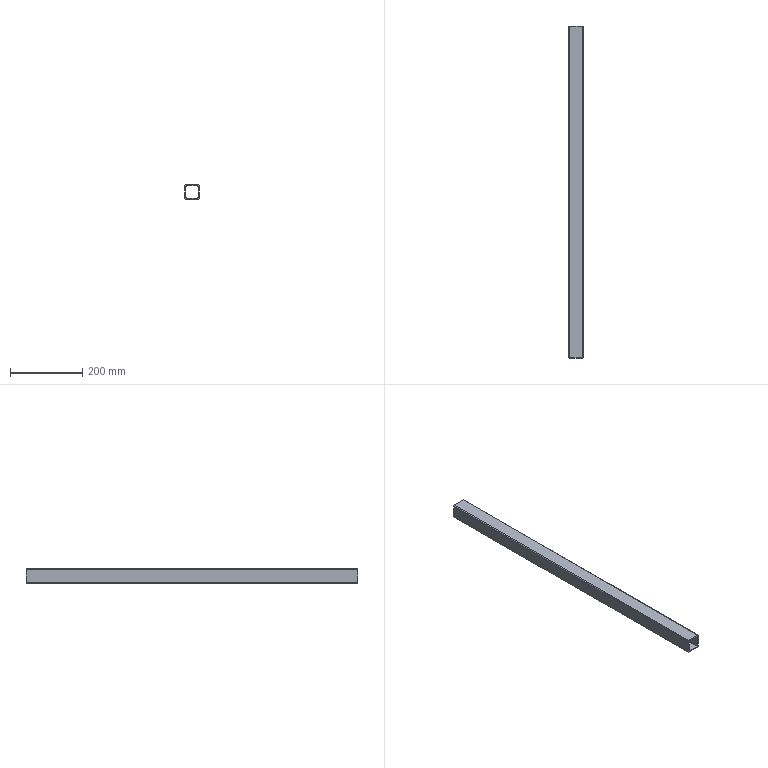Part | STEP file | SynoNew-0304-043 | 1 solid | 18 faces | box 40 x 920 x 40 mm | volume 408480 mm3 | plane 10 | cylinder 8 | commonest cylinder face diameters 4 x8
STEP:
#1=CARTESIAN_POINT('',(-18.,-460.,0.));
#2=VERTEX_POINT('',#1);
#3=CARTESIAN_POINT('',(-20.,-460.,2.));
#4=VERTEX_POINT('',#3);
#5=CARTESIAN_POINT('',(-18.,-460.,2.));
#6=DIRECTION('',(0.,1.,0.));
#7=DIRECTION('',(-0.7071,0.,-0.7071));
#8=AXIS2_PLACEMENT_3D('',#5,#6,#7);
#9=CIRCLE('',#8,2.);
#10=EDGE_CURVE('',#2,#4,#9,.T.);
#11=ORIENTED_EDGE('',*,*,#10,.T.);
#12=CARTESIAN_POINT('',(-20.,460.,2.));
#13=VERTEX_POINT('',#12);
#14=CARTESIAN_POINT('',(-20.,230.,2.));
#15=DIRECTION('',(0.,1.,0.));
#16=VECTOR('',#15,10.);
#17=LINE('',#14,#16);
#18=EDGE_CURVE('',#4,#13,#17,.T.);
#19=ORIENTED_EDGE('',*,*,#18,.T.);
#20=CARTESIAN_POINT('',(-18.,460.,0.));
#21=VERTEX_POINT('',#20);
#22=CARTESIAN_POINT('',(-18.,460.,2.));
#23=DIRECTION('',(0.,-1.,0.));
#24=DIRECTION('',(-0.7071,0.,-0.7071));
#25=AXIS2_PLACEMENT_3D('',#22,#23,#24);
#26=CIRCLE('',#25,2.);
#27=EDGE_CURVE('',#13,#21,#26,.T.);
#28=ORIENTED_EDGE('',*,*,#27,.T.);
#29=CARTESIAN_POINT('',(-18.,230.,0.));
#30=DIRECTION('',(0.,-1.,0.));
#31=VECTOR('',#30,10.);
#32=LINE('',#29,#31);
#33=EDGE_CURVE('',#21,#2,#32,.T.);
#34=ORIENTED_EDGE('',*,*,#33,.T.);
#35=EDGE_LOOP('',(#11,#19,#28,#34));
#36=FACE_OUTER_BOUND('',#35,.T.);
#37=CARTESIAN_POINT('',(-18.,230.,2.));
#38=DIRECTION('',(0.,-1.,0.));
#39=DIRECTION('',(-0.7071,0.,-0.7071));
#40=AXIS2_PLACEMENT_3D('',#37,#38,#39);
#41=CYLINDRICAL_SURFACE('',#40,2.);
#42=ADVANCED_FACE('',(#36),#41,.T.);
#43=ORIENTED_EDGE('',*,*,#33,.F.);
#44=CARTESIAN_POINT('',(18.,460.,0.));
#45=VERTEX_POINT('',#44);
#46=CARTESIAN_POINT('',(20.,460.,0.));
#47=DIRECTION('',(-1.,0.,0.));
#48=VECTOR('',#47,10.);
#49=LINE('',#46,#48);
#50=EDGE_CURVE('',#45,#21,#49,.T.);
#51=ORIENTED_EDGE('',*,*,#50,.F.);
#52=CARTESIAN_POINT('',(18.,-460.,0.));
#53=VERTEX_POINT('',#52);
#54=CARTESIAN_POINT('',(18.,-230.,0.));
#55=DIRECTION('',(0.,1.,0.));
#56=VECTOR('',#55,10.);
#57=LINE('',#54,#56);
#58=EDGE_CURVE('',#53,#45,#57,.T.);
#59=ORIENTED_EDGE('',*,*,#58,.F.);
#60=CARTESIAN_POINT('',(-20.,-460.,0.));
#61=DIRECTION('',(1.,0.,0.));
#62=VECTOR('',#61,10.);
#63=LINE('',#60,#62);
#64=EDGE_CURVE('',#2,#53,#63,.T.);
#65=ORIENTED_EDGE('',*,*,#64,.F.);
#66=EDGE_LOOP('',(#43,#51,#59,#65));
#67=FACE_OUTER_BOUND('',#66,.T.);
#68=CARTESIAN_POINT('',(0.,0.,0.));
#69=DIRECTION('',(0.,0.,1.));
#70=DIRECTION('',(1.,0.,0.));
#71=AXIS2_PLACEMENT_3D('',#68,#69,#70);
#72=PLANE('',#71);
#73=ADVANCED_FACE('',(#67),#72,.F.);
#74=ORIENTED_EDGE('',*,*,#27,.F.);
#75=CARTESIAN_POINT('',(-20.,460.,38.));
#76=VERTEX_POINT('',#75);
#77=CARTESIAN_POINT('',(-20.,460.,0.));
#78=DIRECTION('',(0.,0.,1.));
#79=VECTOR('',#78,10.);
#80=LINE('',#77,#79);
#81=EDGE_CURVE('',#13,#76,#80,.T.);
#82=ORIENTED_EDGE('',*,*,#81,.T.);
#83=CARTESIAN_POINT('',(-18.,460.,40.));
#84=VERTEX_POINT('',#83);
#85=CARTESIAN_POINT('',(-18.,460.,38.));
#86=DIRECTION('',(0.,-1.,0.));
#87=DIRECTION('',(-0.7071,0.,0.7071));
#88=AXIS2_PLACEMENT_3D('',#85,#86,#87);
#89=CIRCLE('',#88,2.);
#90=EDGE_CURVE('',#84,#76,#89,.T.);
#91=ORIENTED_EDGE('',*,*,#90,.F.);
#92=CARTESIAN_POINT('',(18.,460.,40.));
#93=VERTEX_POINT('',#92);
#94=CARTESIAN_POINT('',(20.,460.,40.));
#95=DIRECTION('',(-1.,0.,0.));
#96=VECTOR('',#95,10.);
#97=LINE('',#94,#96);
#98=EDGE_CURVE('',#93,#84,#97,.T.);
#99=ORIENTED_EDGE('',*,*,#98,.F.);
#100=CARTESIAN_POINT('',(20.,460.,38.));
#101=VERTEX_POINT('',#100);
#102=CARTESIAN_POINT('',(18.,460.,38.));
#103=DIRECTION('',(0.,-1.,0.));
#104=DIRECTION('',(0.7071,0.,0.7071));
#105=AXIS2_PLACEMENT_3D('',#102,#103,#104);
#106=CIRCLE('',#105,2.);
#107=EDGE_CURVE('',#101,#93,#106,.T.);
#108=ORIENTED_EDGE('',*,*,#107,.F.);
#109=CARTESIAN_POINT('',(20.,460.,2.));
#110=VERTEX_POINT('',#109);
#111=CARTESIAN_POINT('',(20.,460.,0.));
#112=DIRECTION('',(0.,0.,1.));
#113=VECTOR('',#112,10.);
#114=LINE('',#111,#113);
#115=EDGE_CURVE('',#110,#101,#114,.T.);
#116=ORIENTED_EDGE('',*,*,#115,.F.);
#117=CARTESIAN_POINT('',(18.,460.,2.));
#118=DIRECTION('',(0.,-1.,0.));
#119=DIRECTION('',(0.7071,0.,-0.7071));
#120=AXIS2_PLACEMENT_3D('',#117,#118,#119);
#121=CIRCLE('',#120,2.);
#122=EDGE_CURVE('',#45,#110,#121,.T.);
#123=ORIENTED_EDGE('',*,*,#122,.F.);
#124=ORIENTED_EDGE('',*,*,#50,.T.);
#125=EDGE_LOOP('',(#74,#82,#91,#99,#108,#116,#123,#124));
#126=FACE_OUTER_BOUND('',#125,.T.);
#127=CARTESIAN_POINT('',(17.,460.,5.));
#128=VERTEX_POINT('',#127);
#129=CARTESIAN_POINT('',(17.,460.,35.));
#130=VERTEX_POINT('',#129);
#131=CARTESIAN_POINT('',(17.,460.,1.5));
#132=DIRECTION('',(0.,0.,1.));
#133=VECTOR('',#132,10.);
#134=LINE('',#131,#133);
#135=EDGE_CURVE('',#128,#130,#134,.T.);
#136=ORIENTED_EDGE('',*,*,#135,.T.);
#137=CARTESIAN_POINT('',(15.,460.,37.));
#138=VERTEX_POINT('',#137);
#139=CARTESIAN_POINT('',(15.,460.,35.));
#140=DIRECTION('',(0.,1.,0.));
#141=DIRECTION('',(0.7071,0.,0.7071));
#142=AXIS2_PLACEMENT_3D('',#139,#140,#141);
#143=CIRCLE('',#142,2.);
#144=EDGE_CURVE('',#138,#130,#143,.T.);
#145=ORIENTED_EDGE('',*,*,#144,.F.);
#146=CARTESIAN_POINT('',(-15.,460.,37.));
#147=VERTEX_POINT('',#146);
#148=CARTESIAN_POINT('',(18.5,460.,37.));
#149=DIRECTION('',(-1.,0.,0.));
#150=VECTOR('',#149,10.);
#151=LINE('',#148,#150);
#152=EDGE_CURVE('',#138,#147,#151,.T.);
#153=ORIENTED_EDGE('',*,*,#152,.T.);
#154=CARTESIAN_POINT('',(-17.,460.,35.));
#155=VERTEX_POINT('',#154);
#156=CARTESIAN_POINT('',(-15.,460.,35.));
#157=DIRECTION('',(0.,1.,0.));
#158=DIRECTION('',(-0.7071,0.,0.7071));
#159=AXIS2_PLACEMENT_3D('',#156,#157,#158);
#160=CIRCLE('',#159,2.);
#161=EDGE_CURVE('',#155,#147,#160,.T.);
#162=ORIENTED_EDGE('',*,*,#161,.F.);
#163=CARTESIAN_POINT('',(-17.,460.,5.));
#164=VERTEX_POINT('',#163);
#165=CARTESIAN_POINT('',(-17.,460.,18.5));
#166=DIRECTION('',(0.,0.,-1.));
#167=VECTOR('',#166,10.);
#168=LINE('',#165,#167);
#169=EDGE_CURVE('',#155,#164,#168,.T.);
#170=ORIENTED_EDGE('',*,*,#169,.T.);
#171=CARTESIAN_POINT('',(-15.,460.,3.));
#172=VERTEX_POINT('',#171);
#173=CARTESIAN_POINT('',(-15.,460.,5.));
#174=DIRECTION('',(0.,1.,0.));
#175=DIRECTION('',(-0.7071,0.,-0.7071));
#176=AXIS2_PLACEMENT_3D('',#173,#174,#175);
#177=CIRCLE('',#176,2.);
#178=EDGE_CURVE('',#172,#164,#177,.T.);
#179=ORIENTED_EDGE('',*,*,#178,.F.);
#180=CARTESIAN_POINT('',(15.,460.,3.));
#181=VERTEX_POINT('',#180);
#182=CARTESIAN_POINT('',(1.5,460.,3.));
#183=DIRECTION('',(1.,0.,0.));
#184=VECTOR('',#183,10.);
#185=LINE('',#182,#184);
#186=EDGE_CURVE('',#172,#181,#185,.T.);
#187=ORIENTED_EDGE('',*,*,#186,.T.);
#188=CARTESIAN_POINT('',(15.,460.,5.));
#189=DIRECTION('',(0.,1.,0.));
#190=DIRECTION('',(0.7071,0.,-0.7071));
#191=AXIS2_PLACEMENT_3D('',#188,#189,#190);
#192=CIRCLE('',#191,2.);
#193=EDGE_CURVE('',#128,#181,#192,.T.);
#194=ORIENTED_EDGE('',*,*,#193,.F.);
#195=EDGE_LOOP('',(#136,#145,#153,#162,#170,#179,#187,#194));
#196=FACE_BOUND('',#195,.T.);
#197=CARTESIAN_POINT('',(20.,460.,0.));
#198=DIRECTION('',(0.,1.,0.));
#199=DIRECTION('',(-1.,0.,0.));
#200=AXIS2_PLACEMENT_3D('',#197,#198,#199);
#201=PLANE('',#200);
#202=ADVANCED_FACE('',(#126,#196),#201,.T.);
#203=ORIENTED_EDGE('',*,*,#178,.T.);
#204=CARTESIAN_POINT('',(-17.,-460.,5.));
#205=VERTEX_POINT('',#204);
#206=CARTESIAN_POINT('',(-17.,460.,5.));
#207=DIRECTION('',(0.,-1.,0.));
#208=VECTOR('',#207,10.);
#209=LINE('',#206,#208);
#210=EDGE_CURVE('',#164,#205,#209,.T.);
#211=ORIENTED_EDGE('',*,*,#210,.T.);
#212=CARTESIAN_POINT('',(-15.,-460.,3.));
#213=VERTEX_POINT('',#212);
#214=CARTESIAN_POINT('',(-15.,-460.,5.));
#215=DIRECTION('',(0.,-1.,0.));
#216=DIRECTION('',(-0.7071,0.,-0.7071));
#217=AXIS2_PLACEMENT_3D('',#214,#215,#216);
#218=CIRCLE('',#217,2.);
#219=EDGE_CURVE('',#205,#213,#218,.T.);
#220=ORIENTED_EDGE('',*,*,#219,.T.);
#221=CARTESIAN_POINT('',(-15.,460.,3.));
#222=DIRECTION('',(0.,1.,0.));
#223=VECTOR('',#222,10.);
#224=LINE('',#221,#223);
#225=EDGE_CURVE('',#213,#172,#224,.T.);
#226=ORIENTED_EDGE('',*,*,#225,.T.);
#227=EDGE_LOOP('',(#203,#211,#220,#226));
#228=FACE_OUTER_BOUND('',#227,.T.);
#229=CARTESIAN_POINT('',(-15.,460.,5.));
#230=DIRECTION('',(0.,-1.,0.));
#231=DIRECTION('',(-0.7071,0.,-0.7071));
#232=AXIS2_PLACEMENT_3D('',#229,#230,#231);
#233=CYLINDRICAL_SURFACE('',#232,2.);
#234=ADVANCED_FACE('',(#228),#233,.F.);
#235=ORIENTED_EDGE('',*,*,#210,.F.);
#236=ORIENTED_EDGE('',*,*,#169,.F.);
#237=CARTESIAN_POINT('',(-17.,-460.,35.));
#238=VERTEX_POINT('',#237);
#239=CARTESIAN_POINT('',(-17.,460.,35.));
#240=DIRECTION('',(0.,1.,0.));
#241=VECTOR('',#240,10.);
#242=LINE('',#239,#241);
#243=EDGE_CURVE('',#238,#155,#242,.T.);
#244=ORIENTED_EDGE('',*,*,#243,.F.);
#245=CARTESIAN_POINT('',(-17.,-460.,18.5));
#246=DIRECTION('',(0.,0.,1.));
#247=VECTOR('',#246,10.);
#248=LINE('',#245,#247);
#249=EDGE_CURVE('',#205,#238,#248,.T.);
#250=ORIENTED_EDGE('',*,*,#249,.F.);
#251=EDGE_LOOP('',(#235,#236,#244,#250));
#252=FACE_OUTER_BOUND('',#251,.T.);
#253=CARTESIAN_POINT('',(-17.,460.,37.));
#254=DIRECTION('',(-1.,0.,0.));
#255=DIRECTION('',(0.,0.,-1.));
#256=AXIS2_PLACEMENT_3D('',#253,#254,#255);
#257=PLANE('',#256);
#258=ADVANCED_FACE('',(#252),#257,.F.);
#259=ORIENTED_EDGE('',*,*,#161,.T.);
#260=CARTESIAN_POINT('',(-15.,-460.,37.));
#261=VERTEX_POINT('',#260);
#262=CARTESIAN_POINT('',(-15.,460.,37.));
#263=DIRECTION('',(0.,-1.,0.));
#264=VECTOR('',#263,10.);
#265=LINE('',#262,#264);
#266=EDGE_CURVE('',#147,#261,#265,.T.);
#267=ORIENTED_EDGE('',*,*,#266,.T.);
#268=CARTESIAN_POINT('',(-15.,-460.,35.));
#269=DIRECTION('',(0.,-1.,0.));
#270=DIRECTION('',(-0.7071,0.,0.7071));
#271=AXIS2_PLACEMENT_3D('',#268,#269,#270);
#272=CIRCLE('',#271,2.);
#273=EDGE_CURVE('',#261,#238,#272,.T.);
#274=ORIENTED_EDGE('',*,*,#273,.T.);
#275=ORIENTED_EDGE('',*,*,#243,.T.);
#276=EDGE_LOOP('',(#259,#267,#274,#275));
#277=FACE_OUTER_BOUND('',#276,.T.);
#278=CARTESIAN_POINT('',(-15.,460.,35.));
#279=DIRECTION('',(0.,-1.,0.));
#280=DIRECTION('',(-0.7071,0.,0.7071));
#281=AXIS2_PLACEMENT_3D('',#278,#279,#280);
#282=CYLINDRICAL_SURFACE('',#281,2.);
#283=ADVANCED_FACE('',(#277),#282,.F.);
#284=ORIENTED_EDGE('',*,*,#266,.F.);
#285=ORIENTED_EDGE('',*,*,#152,.F.);
#286=CARTESIAN_POINT('',(15.,-460.,37.));
#287=VERTEX_POINT('',#286);
#288=CARTESIAN_POINT('',(15.,460.,37.));
#289=DIRECTION('',(0.,1.,0.));
#290=VECTOR('',#289,10.);
#291=LINE('',#288,#290);
#292=EDGE_CURVE('',#287,#138,#291,.T.);
#293=ORIENTED_EDGE('',*,*,#292,.F.);
#294=CARTESIAN_POINT('',(-1.5,-460.,37.));
#295=DIRECTION('',(1.,0.,0.));
#296=VECTOR('',#295,10.);
#297=LINE('',#294,#296);
#298=EDGE_CURVE('',#261,#287,#297,.T.);
#299=ORIENTED_EDGE('',*,*,#298,.F.);
#300=EDGE_LOOP('',(#284,#285,#293,#299));
#301=FACE_OUTER_BOUND('',#300,.T.);
#302=CARTESIAN_POINT('',(17.,460.,37.));
#303=DIRECTION('',(0.,0.,1.));
#304=DIRECTION('',(-1.,0.,0.));
#305=AXIS2_PLACEMENT_3D('',#302,#303,#304);
#306=PLANE('',#305);
#307=ADVANCED_FACE('',(#301),#306,.F.);
#308=CARTESIAN_POINT('',(-20.,-460.,38.));
#309=VERTEX_POINT('',#308);
#310=CARTESIAN_POINT('',(-18.,-460.,40.));
#311=VERTEX_POINT('',#310);
#312=CARTESIAN_POINT('',(-18.,-460.,38.));
#313=DIRECTION('',(0.,1.,0.));
#314=DIRECTION('',(-0.7071,0.,0.7071));
#315=AXIS2_PLACEMENT_3D('',#312,#313,#314);
#316=CIRCLE('',#315,2.);
#317=EDGE_CURVE('',#309,#311,#316,.T.);
#318=ORIENTED_EDGE('',*,*,#317,.T.);
#319=CARTESIAN_POINT('',(-18.,230.,40.));
#320=DIRECTION('',(0.,1.,0.));
#321=VECTOR('',#320,10.);
#322=LINE('',#319,#321);
#323=EDGE_CURVE('',#311,#84,#322,.T.);
#324=ORIENTED_EDGE('',*,*,#323,.T.);
#325=ORIENTED_EDGE('',*,*,#90,.T.);
#326=CARTESIAN_POINT('',(-20.,230.,38.));
#327=DIRECTION('',(0.,-1.,0.));
#328=VECTOR('',#327,10.);
#329=LINE('',#326,#328);
#330=EDGE_CURVE('',#76,#309,#329,.T.);
#331=ORIENTED_EDGE('',*,*,#330,.T.);
#332=EDGE_LOOP('',(#318,#324,#325,#331));
#333=FACE_OUTER_BOUND('',#332,.T.);
#334=CARTESIAN_POINT('',(-18.,230.,38.));
#335=DIRECTION('',(0.,-1.,0.));
#336=DIRECTION('',(-0.7071,0.,0.7071));
#337=AXIS2_PLACEMENT_3D('',#334,#335,#336);
#338=CYLINDRICAL_SURFACE('',#337,2.);
#339=ADVANCED_FACE('',(#333),#338,.T.);
#340=ORIENTED_EDGE('',*,*,#323,.F.);
#341=CARTESIAN_POINT('',(18.,-460.,40.));
#342=VERTEX_POINT('',#341);
#343=CARTESIAN_POINT('',(-20.,-460.,40.));
#344=DIRECTION('',(1.,0.,0.));
#345=VECTOR('',#344,10.);
#346=LINE('',#343,#345);
#347=EDGE_CURVE('',#311,#342,#346,.T.);
#348=ORIENTED_EDGE('',*,*,#347,.T.);
#349=CARTESIAN_POINT('',(18.,-230.,40.));
#350=DIRECTION('',(0.,-1.,0.));
#351=VECTOR('',#350,10.);
#352=LINE('',#349,#351);
#353=EDGE_CURVE('',#93,#342,#352,.T.);
#354=ORIENTED_EDGE('',*,*,#353,.F.);
#355=ORIENTED_EDGE('',*,*,#98,.T.);
#356=EDGE_LOOP('',(#340,#348,#354,#355));
#357=FACE_OUTER_BOUND('',#356,.T.);
#358=CARTESIAN_POINT('',(0.,0.,40.));
#359=DIRECTION('',(0.,0.,1.));
#360=DIRECTION('',(1.,0.,0.));
#361=AXIS2_PLACEMENT_3D('',#358,#359,#360);
#362=PLANE('',#361);
#363=ADVANCED_FACE('',(#357),#362,.T.);
#364=ORIENTED_EDGE('',*,*,#10,.F.);
#365=ORIENTED_EDGE('',*,*,#64,.T.);
#366=CARTESIAN_POINT('',(20.,-460.,2.));
#367=VERTEX_POINT('',#366);
#368=CARTESIAN_POINT('',(18.,-460.,2.));
#369=DIRECTION('',(0.,1.,0.));
#370=DIRECTION('',(0.7071,0.,-0.7071));
#371=AXIS2_PLACEMENT_3D('',#368,#369,#370);
#372=CIRCLE('',#371,2.);
#373=EDGE_CURVE('',#367,#53,#372,.T.);
#374=ORIENTED_EDGE('',*,*,#373,.F.);
#375=CARTESIAN_POINT('',(20.,-460.,38.));
#376=VERTEX_POINT('',#375);
#377=CARTESIAN_POINT('',(20.,-460.,0.));
#378=DIRECTION('',(0.,0.,1.));
#379=VECTOR('',#378,10.);
#380=LINE('',#377,#379);
#381=EDGE_CURVE('',#367,#376,#380,.T.);
#382=ORIENTED_EDGE('',*,*,#381,.T.);
#383=CARTESIAN_POINT('',(18.,-460.,38.));
#384=DIRECTION('',(0.,1.,0.));
#385=DIRECTION('',(0.7071,0.,0.7071));
#386=AXIS2_PLACEMENT_3D('',#383,#384,#385);
#387=CIRCLE('',#386,2.);
#388=EDGE_CURVE('',#342,#376,#387,.T.);
#389=ORIENTED_EDGE('',*,*,#388,.F.);
#390=ORIENTED_EDGE('',*,*,#347,.F.);
#391=ORIENTED_EDGE('',*,*,#317,.F.);
#392=CARTESIAN_POINT('',(-20.,-460.,0.));
#393=DIRECTION('',(0.,0.,1.));
#394=VECTOR('',#393,10.);
#395=LINE('',#392,#394);
#396=EDGE_CURVE('',#4,#309,#395,.T.);
#397=ORIENTED_EDGE('',*,*,#396,.F.);
#398=EDGE_LOOP('',(#364,#365,#374,#382,#389,#390,#391,#397));
#399=FACE_OUTER_BOUND('',#398,.T.);
#400=CARTESIAN_POINT('',(17.,-460.,35.));
#401=VERTEX_POINT('',#400);
#402=CARTESIAN_POINT('',(17.,-460.,5.));
#403=VERTEX_POINT('',#402);
#404=CARTESIAN_POINT('',(17.,-460.,1.5));
#405=DIRECTION('',(0.,0.,-1.));
#406=VECTOR('',#405,10.);
#407=LINE('',#404,#406);
#408=EDGE_CURVE('',#401,#403,#407,.T.);
#409=ORIENTED_EDGE('',*,*,#408,.T.);
#410=CARTESIAN_POINT('',(15.,-460.,3.));
#411=VERTEX_POINT('',#410);
#412=CARTESIAN_POINT('',(15.,-460.,5.));
#413=DIRECTION('',(0.,-1.,0.));
#414=DIRECTION('',(0.7071,0.,-0.7071));
#415=AXIS2_PLACEMENT_3D('',#412,#413,#414);
#416=CIRCLE('',#415,2.);
#417=EDGE_CURVE('',#411,#403,#416,.T.);
#418=ORIENTED_EDGE('',*,*,#417,.F.);
#419=CARTESIAN_POINT('',(-18.5,-460.,3.));
#420=DIRECTION('',(-1.,0.,0.));
#421=VECTOR('',#420,10.);
#422=LINE('',#419,#421);
#423=EDGE_CURVE('',#411,#213,#422,.T.);
#424=ORIENTED_EDGE('',*,*,#423,.T.);
#425=ORIENTED_EDGE('',*,*,#219,.F.);
#426=ORIENTED_EDGE('',*,*,#249,.T.);
#427=ORIENTED_EDGE('',*,*,#273,.F.);
#428=ORIENTED_EDGE('',*,*,#298,.T.);
#429=CARTESIAN_POINT('',(15.,-460.,35.));
#430=DIRECTION('',(0.,-1.,0.));
#431=DIRECTION('',(0.7071,0.,0.7071));
#432=AXIS2_PLACEMENT_3D('',#429,#430,#431);
#433=CIRCLE('',#432,2.);
#434=EDGE_CURVE('',#401,#287,#433,.T.);
#435=ORIENTED_EDGE('',*,*,#434,.F.);
#436=EDGE_LOOP('',(#409,#418,#424,#425,#426,#427,#428,#435));
#437=FACE_BOUND('',#436,.T.);
#438=CARTESIAN_POINT('',(-20.,-460.,0.));
#439=DIRECTION('',(0.,-1.,0.));
#440=DIRECTION('',(1.,0.,0.));
#441=AXIS2_PLACEMENT_3D('',#438,#439,#440);
#442=PLANE('',#441);
#443=ADVANCED_FACE('',(#399,#437),#442,.T.);
#444=ORIENTED_EDGE('',*,*,#144,.T.);
#445=CARTESIAN_POINT('',(17.,460.,35.));
#446=DIRECTION('',(0.,-1.,0.));
#447=VECTOR('',#446,10.);
#448=LINE('',#445,#447);
#449=EDGE_CURVE('',#130,#401,#448,.T.);
#450=ORIENTED_EDGE('',*,*,#449,.T.);
#451=ORIENTED_EDGE('',*,*,#434,.T.);
#452=ORIENTED_EDGE('',*,*,#292,.T.);
#453=EDGE_LOOP('',(#444,#450,#451,#452));
#454=FACE_OUTER_BOUND('',#453,.T.);
#455=CARTESIAN_POINT('',(15.,460.,35.));
#456=DIRECTION('',(0.,-1.,0.));
#457=DIRECTION('',(0.7071,0.,0.7071));
#458=AXIS2_PLACEMENT_3D('',#455,#456,#457);
#459=CYLINDRICAL_SURFACE('',#458,2.);
#460=ADVANCED_FACE('',(#454),#459,.F.);
#461=ORIENTED_EDGE('',*,*,#449,.F.);
#462=ORIENTED_EDGE('',*,*,#135,.F.);
#463=CARTESIAN_POINT('',(17.,460.,5.));
#464=DIRECTION('',(0.,1.,0.));
#465=VECTOR('',#464,10.);
#466=LINE('',#463,#465);
#467=EDGE_CURVE('',#403,#128,#466,.T.);
#468=ORIENTED_EDGE('',*,*,#467,.F.);
#469=ORIENTED_EDGE('',*,*,#408,.F.);
#470=EDGE_LOOP('',(#461,#462,#468,#469));
#471=FACE_OUTER_BOUND('',#470,.T.);
#472=CARTESIAN_POINT('',(17.,460.,3.));
#473=DIRECTION('',(1.,0.,0.));
#474=DIRECTION('',(0.,0.,1.));
#475=AXIS2_PLACEMENT_3D('',#472,#473,#474);
#476=PLANE('',#475);
#477=ADVANCED_FACE('',(#471),#476,.F.);
#478=ORIENTED_EDGE('',*,*,#107,.T.);
#479=ORIENTED_EDGE('',*,*,#353,.T.);
#480=ORIENTED_EDGE('',*,*,#388,.T.);
#481=CARTESIAN_POINT('',(20.,-230.,38.));
#482=DIRECTION('',(0.,1.,0.));
#483=VECTOR('',#482,10.);
#484=LINE('',#481,#483);
#485=EDGE_CURVE('',#376,#101,#484,.T.);
#486=ORIENTED_EDGE('',*,*,#485,.T.);
#487=EDGE_LOOP('',(#478,#479,#480,#486));
#488=FACE_OUTER_BOUND('',#487,.T.);
#489=CARTESIAN_POINT('',(18.,-230.,38.));
#490=DIRECTION('',(0.,1.,0.));
#491=DIRECTION('',(0.7071,0.,0.7071));
#492=AXIS2_PLACEMENT_3D('',#489,#490,#491);
#493=CYLINDRICAL_SURFACE('',#492,2.);
#494=ADVANCED_FACE('',(#488),#493,.T.);
#495=ORIENTED_EDGE('',*,*,#485,.F.);
#496=ORIENTED_EDGE('',*,*,#381,.F.);
#497=CARTESIAN_POINT('',(20.,-230.,2.));
#498=DIRECTION('',(0.,-1.,0.));
#499=VECTOR('',#498,10.);
#500=LINE('',#497,#499);
#501=EDGE_CURVE('',#110,#367,#500,.T.);
#502=ORIENTED_EDGE('',*,*,#501,.F.);
#503=ORIENTED_EDGE('',*,*,#115,.T.);
#504=EDGE_LOOP('',(#495,#496,#502,#503));
#505=FACE_OUTER_BOUND('',#504,.T.);
#506=CARTESIAN_POINT('',(20.,-460.,0.));
#507=DIRECTION('',(1.,0.,0.));
#508=DIRECTION('',(0.,1.,0.));
#509=AXIS2_PLACEMENT_3D('',#506,#507,#508);
#510=PLANE('',#509);
#511=ADVANCED_FACE('',(#505),#510,.T.);
#512=ORIENTED_EDGE('',*,*,#122,.T.);
#513=ORIENTED_EDGE('',*,*,#501,.T.);
#514=ORIENTED_EDGE('',*,*,#373,.T.);
#515=ORIENTED_EDGE('',*,*,#58,.T.);
#516=EDGE_LOOP('',(#512,#513,#514,#515));
#517=FACE_OUTER_BOUND('',#516,.T.);
#518=CARTESIAN_POINT('',(18.,-230.,2.));
#519=DIRECTION('',(0.,1.,0.));
#520=DIRECTION('',(0.7071,0.,-0.7071));
#521=AXIS2_PLACEMENT_3D('',#518,#519,#520);
#522=CYLINDRICAL_SURFACE('',#521,2.);
#523=ADVANCED_FACE('',(#517),#522,.T.);
#524=ORIENTED_EDGE('',*,*,#193,.T.);
#525=CARTESIAN_POINT('',(15.,460.,3.));
#526=DIRECTION('',(0.,-1.,0.));
#527=VECTOR('',#526,10.);
#528=LINE('',#525,#527);
#529=EDGE_CURVE('',#181,#411,#528,.T.);
#530=ORIENTED_EDGE('',*,*,#529,.T.);
#531=ORIENTED_EDGE('',*,*,#417,.T.);
#532=ORIENTED_EDGE('',*,*,#467,.T.);
#533=EDGE_LOOP('',(#524,#530,#531,#532));
#534=FACE_OUTER_BOUND('',#533,.T.);
#535=CARTESIAN_POINT('',(15.,460.,5.));
#536=DIRECTION('',(0.,-1.,0.));
#537=DIRECTION('',(0.7071,0.,-0.7071));
#538=AXIS2_PLACEMENT_3D('',#535,#536,#537);
#539=CYLINDRICAL_SURFACE('',#538,2.);
#540=ADVANCED_FACE('',(#534),#539,.F.);
#541=ORIENTED_EDGE('',*,*,#225,.F.);
#542=ORIENTED_EDGE('',*,*,#423,.F.);
#543=ORIENTED_EDGE('',*,*,#529,.F.);
#544=ORIENTED_EDGE('',*,*,#186,.F.);
#545=EDGE_LOOP('',(#541,#542,#543,#544));
#546=FACE_OUTER_BOUND('',#545,.T.);
#547=CARTESIAN_POINT('',(-17.,460.,3.));
#548=DIRECTION('',(0.,0.,-1.));
#549=DIRECTION('',(1.,0.,0.));
#550=AXIS2_PLACEMENT_3D('',#547,#548,#549);
#551=PLANE('',#550);
#552=ADVANCED_FACE('',(#546),#551,.F.);
#553=ORIENTED_EDGE('',*,*,#18,.F.);
#554=ORIENTED_EDGE('',*,*,#396,.T.);
#555=ORIENTED_EDGE('',*,*,#330,.F.);
#556=ORIENTED_EDGE('',*,*,#81,.F.);
#557=EDGE_LOOP('',(#553,#554,#555,#556));
#558=FACE_OUTER_BOUND('',#557,.T.);
#559=CARTESIAN_POINT('',(-20.,460.,0.));
#560=DIRECTION('',(-1.,0.,0.));
#561=DIRECTION('',(0.,-1.,0.));
#562=AXIS2_PLACEMENT_3D('',#559,#560,#561);
#563=PLANE('',#562);
#564=ADVANCED_FACE('',(#558),#563,.T.);
#565=CLOSED_SHELL('',(#42,#73,#202,#234,#258,#283,#307,#339,#363,#443,#460,#477,#494,#511,#523,#540,#552,#564));
#566=MANIFOLD_SOLID_BREP('',#565);
#567=(LENGTH_UNIT()NAMED_UNIT(*)SI_UNIT(.MILLI.,.METRE.));
#568=UNCERTAINTY_MEASURE_WITH_UNIT(LENGTH_MEASURE(0.01),#567,'','');
#569=(NAMED_UNIT(*)PLANE_ANGLE_UNIT()SI_UNIT($,.RADIAN.));
#570=(NAMED_UNIT(*)SI_UNIT($,.STERADIAN.)SOLID_ANGLE_UNIT());
#571=(GEOMETRIC_REPRESENTATION_CONTEXT(3)GLOBAL_UNCERTAINTY_ASSIGNED_CONTEXT((#568))GLOBAL_UNIT_ASSIGNED_CONTEXT((#567,#569,#570))REPRESENTATION_CONTEXT('',''));
#572=ADVANCED_BREP_SHAPE_REPRESENTATION('',(#566),#571);